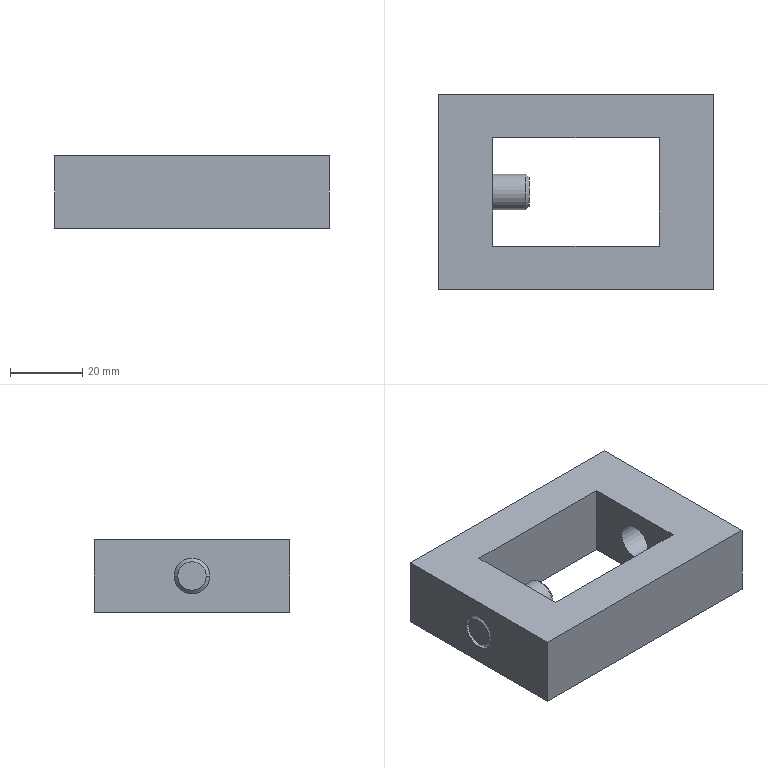Part | SolidWorks | features MirrorStock 1 | 2 solids | 22 faces | box 76 x 54 x 20 mm | volume 53995 mm3 | plane 12 | cylinder 6 | cone 4 | commonest cylinder face diameters 9.9 x4 10.2 x2
STEP:
#1=CARTESIAN_POINT('',(23.,0.,-5.1));
#2=VERTEX_POINT('',#1);
#3=CARTESIAN_POINT('',(23.,0.,5.1));
#4=VERTEX_POINT('',#3);
#5=CARTESIAN_POINT('',(23.,0.,0.));
#6=DIRECTION('',(1.,0.,0.));
#7=DIRECTION('',(0.,0.,-1.));
#8=AXIS2_PLACEMENT_3D('',#5,#6,#7);
#9=CIRCLE('',#8,5.1);
#10=EDGE_CURVE('',#2,#4,#9,.T.);
#11=ORIENTED_EDGE('',*,*,#10,.F.);
#12=CARTESIAN_POINT('',(38.,0.,-5.1));
#13=VERTEX_POINT('',#12);
#14=CARTESIAN_POINT('',(38.,0.,-5.1));
#15=DIRECTION('',(1.,0.,0.));
#16=VECTOR('',#15,1000.);
#17=LINE('',#14,#16);
#18=EDGE_CURVE('',#2,#13,#17,.T.);
#19=ORIENTED_EDGE('',*,*,#18,.T.);
#20=CARTESIAN_POINT('',(38.,0.,5.1));
#21=VERTEX_POINT('',#20);
#22=CARTESIAN_POINT('',(38.,0.,0.));
#23=DIRECTION('',(-1.,0.,0.));
#24=DIRECTION('',(0.,0.,1.));
#25=AXIS2_PLACEMENT_3D('',#22,#23,#24);
#26=CIRCLE('',#25,5.1);
#27=EDGE_CURVE('',#21,#13,#26,.T.);
#28=ORIENTED_EDGE('',*,*,#27,.F.);
#29=CARTESIAN_POINT('',(38.,0.,5.1));
#30=DIRECTION('',(1.,0.,0.));
#31=VECTOR('',#30,1000.);
#32=LINE('',#29,#31);
#33=EDGE_CURVE('',#4,#21,#32,.T.);
#34=ORIENTED_EDGE('',*,*,#33,.F.);
#35=EDGE_LOOP('',(#11,#19,#28,#34));
#36=FACE_OUTER_BOUND('',#35,.T.);
#37=CARTESIAN_POINT('',(38.,0.,0.));
#38=DIRECTION('',(1.,0.,0.));
#39=DIRECTION('',(0.,0.,1.));
#40=AXIS2_PLACEMENT_3D('',#37,#38,#39);
#41=CYLINDRICAL_SURFACE('',#40,5.1);
#42=ADVANCED_FACE('',(#36),#41,.F.);
#43=CARTESIAN_POINT('',(-23.,4.95,0.));
#44=VERTEX_POINT('',#43);
#45=CARTESIAN_POINT('',(-23.,-4.95,0.));
#46=VERTEX_POINT('',#45);
#47=CARTESIAN_POINT('',(-23.,0.,0.));
#48=DIRECTION('',(-1.,0.,0.));
#49=DIRECTION('',(0.,0.,1.));
#50=AXIS2_PLACEMENT_3D('',#47,#48,#49);
#51=CIRCLE('',#50,4.95);
#52=EDGE_CURVE('',#44,#46,#51,.T.);
#53=ORIENTED_EDGE('',*,*,#52,.F.);
#54=CARTESIAN_POINT('',(-38.,4.95,0.));
#55=VERTEX_POINT('',#54);
#56=CARTESIAN_POINT('',(-18.,4.95,0.));
#57=DIRECTION('',(-1.,0.,0.));
#58=VECTOR('',#57,1000.);
#59=LINE('',#56,#58);
#60=EDGE_CURVE('',#44,#55,#59,.T.);
#61=ORIENTED_EDGE('',*,*,#60,.T.);
#62=CARTESIAN_POINT('',(-38.,-4.95,0.));
#63=VERTEX_POINT('',#62);
#64=CARTESIAN_POINT('',(-38.,0.,0.));
#65=DIRECTION('',(1.,0.,0.));
#66=DIRECTION('',(0.,-1.,0.));
#67=AXIS2_PLACEMENT_3D('',#64,#65,#66);
#68=CIRCLE('',#67,4.95);
#69=EDGE_CURVE('',#63,#55,#68,.T.);
#70=ORIENTED_EDGE('',*,*,#69,.F.);
#71=CARTESIAN_POINT('',(-18.,-4.95,0.));
#72=DIRECTION('',(-1.,0.,0.));
#73=VECTOR('',#72,1000.);
#74=LINE('',#71,#73);
#75=EDGE_CURVE('',#46,#63,#74,.T.);
#76=ORIENTED_EDGE('',*,*,#75,.F.);
#77=EDGE_LOOP('',(#53,#61,#70,#76));
#78=FACE_OUTER_BOUND('',#77,.T.);
#79=CARTESIAN_POINT('',(-18.,0.,0.));
#80=DIRECTION('',(-1.,0.,0.));
#81=DIRECTION('',(0.,-1.,0.));
#82=AXIS2_PLACEMENT_3D('',#79,#80,#81);
#83=CYLINDRICAL_SURFACE('',#82,4.95);
#84=ADVANCED_FACE('',(#78),#83,.F.);
#85=CARTESIAN_POINT('',(38.,-27.,-10.));
#86=VERTEX_POINT('',#85);
#87=CARTESIAN_POINT('',(38.,27.,-10.));
#88=VERTEX_POINT('',#87);
#89=CARTESIAN_POINT('',(38.,-27.,-10.));
#90=DIRECTION('',(0.,1.,0.));
#91=VECTOR('',#90,1000.);
#92=LINE('',#89,#91);
#93=EDGE_CURVE('',#86,#88,#92,.T.);
#94=ORIENTED_EDGE('',*,*,#93,.F.);
#95=CARTESIAN_POINT('',(-38.,-27.,-10.));
#96=VERTEX_POINT('',#95);
#97=CARTESIAN_POINT('',(-38.,-27.,-10.));
#98=DIRECTION('',(1.,0.,0.));
#99=VECTOR('',#98,1000.);
#100=LINE('',#97,#99);
#101=EDGE_CURVE('',#96,#86,#100,.T.);
#102=ORIENTED_EDGE('',*,*,#101,.F.);
#103=CARTESIAN_POINT('',(-38.,27.,-10.));
#104=VERTEX_POINT('',#103);
#105=CARTESIAN_POINT('',(-38.,-27.,-10.));
#106=DIRECTION('',(0.,-1.,0.));
#107=VECTOR('',#106,1000.);
#108=LINE('',#105,#107);
#109=EDGE_CURVE('',#104,#96,#108,.T.);
#110=ORIENTED_EDGE('',*,*,#109,.F.);
#111=CARTESIAN_POINT('',(-38.,27.,-10.));
#112=DIRECTION('',(-1.,0.,0.));
#113=VECTOR('',#112,1000.);
#114=LINE('',#111,#113);
#115=EDGE_CURVE('',#88,#104,#114,.T.);
#116=ORIENTED_EDGE('',*,*,#115,.F.);
#117=EDGE_LOOP('',(#94,#102,#110,#116));
#118=FACE_OUTER_BOUND('',#117,.T.);
#119=CARTESIAN_POINT('',(-23.,15.,-10.));
#120=VERTEX_POINT('',#119);
#121=CARTESIAN_POINT('',(-23.,-15.,-10.));
#122=VERTEX_POINT('',#121);
#123=CARTESIAN_POINT('',(-23.,15.,-10.));
#124=DIRECTION('',(0.,-1.,0.));
#125=VECTOR('',#124,1000.);
#126=LINE('',#123,#125);
#127=EDGE_CURVE('',#120,#122,#126,.T.);
#128=ORIENTED_EDGE('',*,*,#127,.T.);
#129=CARTESIAN_POINT('',(23.,-15.,-10.));
#130=VERTEX_POINT('',#129);
#131=CARTESIAN_POINT('',(23.,-15.,-10.));
#132=DIRECTION('',(1.,0.,0.));
#133=VECTOR('',#132,1000.);
#134=LINE('',#131,#133);
#135=EDGE_CURVE('',#122,#130,#134,.T.);
#136=ORIENTED_EDGE('',*,*,#135,.T.);
#137=CARTESIAN_POINT('',(23.,15.,-10.));
#138=VERTEX_POINT('',#137);
#139=CARTESIAN_POINT('',(23.,15.,-10.));
#140=DIRECTION('',(0.,1.,0.));
#141=VECTOR('',#140,1000.);
#142=LINE('',#139,#141);
#143=EDGE_CURVE('',#130,#138,#142,.T.);
#144=ORIENTED_EDGE('',*,*,#143,.T.);
#145=CARTESIAN_POINT('',(23.,15.,-10.));
#146=DIRECTION('',(-1.,0.,0.));
#147=VECTOR('',#146,1000.);
#148=LINE('',#145,#147);
#149=EDGE_CURVE('',#138,#120,#148,.T.);
#150=ORIENTED_EDGE('',*,*,#149,.T.);
#151=EDGE_LOOP('',(#128,#136,#144,#150));
#152=FACE_BOUND('',#151,.T.);
#153=CARTESIAN_POINT('',(0.,0.,-10.));
#154=DIRECTION('',(0.,0.,1.));
#155=DIRECTION('',(-1.,0.,0.));
#156=AXIS2_PLACEMENT_3D('',#153,#154,#155);
#157=PLANE('',#156);
#158=ADVANCED_FACE('',(#118,#152),#157,.F.);
#159=CARTESIAN_POINT('',(38.,-27.,10.));
#160=VERTEX_POINT('',#159);
#161=CARTESIAN_POINT('',(38.,27.,10.));
#162=VERTEX_POINT('',#161);
#163=CARTESIAN_POINT('',(38.,-27.,10.));
#164=DIRECTION('',(0.,1.,0.));
#165=VECTOR('',#164,1000.);
#166=LINE('',#163,#165);
#167=EDGE_CURVE('',#160,#162,#166,.T.);
#168=ORIENTED_EDGE('',*,*,#167,.T.);
#169=CARTESIAN_POINT('',(-38.,27.,10.));
#170=VERTEX_POINT('',#169);
#171=CARTESIAN_POINT('',(-38.,27.,10.));
#172=DIRECTION('',(-1.,0.,0.));
#173=VECTOR('',#172,1000.);
#174=LINE('',#171,#173);
#175=EDGE_CURVE('',#162,#170,#174,.T.);
#176=ORIENTED_EDGE('',*,*,#175,.T.);
#177=CARTESIAN_POINT('',(-38.,-27.,10.));
#178=VERTEX_POINT('',#177);
#179=CARTESIAN_POINT('',(-38.,-27.,10.));
#180=DIRECTION('',(0.,-1.,0.));
#181=VECTOR('',#180,1000.);
#182=LINE('',#179,#181);
#183=EDGE_CURVE('',#170,#178,#182,.T.);
#184=ORIENTED_EDGE('',*,*,#183,.T.);
#185=CARTESIAN_POINT('',(-38.,-27.,10.));
#186=DIRECTION('',(1.,0.,0.));
#187=VECTOR('',#186,1000.);
#188=LINE('',#185,#187);
#189=EDGE_CURVE('',#178,#160,#188,.T.);
#190=ORIENTED_EDGE('',*,*,#189,.T.);
#191=EDGE_LOOP('',(#168,#176,#184,#190));
#192=FACE_OUTER_BOUND('',#191,.T.);
#193=CARTESIAN_POINT('',(23.,15.,10.));
#194=VERTEX_POINT('',#193);
#195=CARTESIAN_POINT('',(-23.,15.,10.));
#196=VERTEX_POINT('',#195);
#197=CARTESIAN_POINT('',(23.,15.,10.));
#198=DIRECTION('',(-1.,0.,0.));
#199=VECTOR('',#198,1000.);
#200=LINE('',#197,#199);
#201=EDGE_CURVE('',#194,#196,#200,.T.);
#202=ORIENTED_EDGE('',*,*,#201,.F.);
#203=CARTESIAN_POINT('',(23.,-15.,10.));
#204=VERTEX_POINT('',#203);
#205=CARTESIAN_POINT('',(23.,15.,10.));
#206=DIRECTION('',(0.,1.,0.));
#207=VECTOR('',#206,1000.);
#208=LINE('',#205,#207);
#209=EDGE_CURVE('',#204,#194,#208,.T.);
#210=ORIENTED_EDGE('',*,*,#209,.F.);
#211=CARTESIAN_POINT('',(-23.,-15.,10.));
#212=VERTEX_POINT('',#211);
#213=CARTESIAN_POINT('',(23.,-15.,10.));
#214=DIRECTION('',(1.,0.,0.));
#215=VECTOR('',#214,1000.);
#216=LINE('',#213,#215);
#217=EDGE_CURVE('',#212,#204,#216,.T.);
#218=ORIENTED_EDGE('',*,*,#217,.F.);
#219=CARTESIAN_POINT('',(-23.,15.,10.));
#220=DIRECTION('',(0.,-1.,0.));
#221=VECTOR('',#220,1000.);
#222=LINE('',#219,#221);
#223=EDGE_CURVE('',#196,#212,#222,.T.);
#224=ORIENTED_EDGE('',*,*,#223,.F.);
#225=EDGE_LOOP('',(#202,#210,#218,#224));
#226=FACE_BOUND('',#225,.T.);
#227=CARTESIAN_POINT('',(0.,0.,10.));
#228=DIRECTION('',(0.,0.,1.));
#229=DIRECTION('',(-1.,0.,0.));
#230=AXIS2_PLACEMENT_3D('',#227,#228,#229);
#231=PLANE('',#230);
#232=ADVANCED_FACE('',(#192,#226),#231,.T.);
#233=ORIENTED_EDGE('',*,*,#27,.T.);
#234=CARTESIAN_POINT('',(38.,0.,0.));
#235=DIRECTION('',(-1.,0.,0.));
#236=DIRECTION('',(0.,0.,1.));
#237=AXIS2_PLACEMENT_3D('',#234,#235,#236);
#238=CIRCLE('',#237,5.1);
#239=EDGE_CURVE('',#13,#21,#238,.T.);
#240=ORIENTED_EDGE('',*,*,#239,.T.);
#241=EDGE_LOOP('',(#233,#240));
#242=FACE_BOUND('',#241,.T.);
#243=ORIENTED_EDGE('',*,*,#167,.F.);
#244=CARTESIAN_POINT('',(38.,-27.,-10.));
#245=DIRECTION('',(0.,0.,1.));
#246=VECTOR('',#245,1000.);
#247=LINE('',#244,#246);
#248=EDGE_CURVE('',#86,#160,#247,.T.);
#249=ORIENTED_EDGE('',*,*,#248,.F.);
#250=ORIENTED_EDGE('',*,*,#93,.T.);
#251=CARTESIAN_POINT('',(38.,27.,-10.));
#252=DIRECTION('',(0.,0.,1.));
#253=VECTOR('',#252,1000.);
#254=LINE('',#251,#253);
#255=EDGE_CURVE('',#88,#162,#254,.T.);
#256=ORIENTED_EDGE('',*,*,#255,.T.);
#257=EDGE_LOOP('',(#243,#249,#250,#256));
#258=FACE_OUTER_BOUND('',#257,.T.);
#259=CARTESIAN_POINT('',(38.,-27.,-10.));
#260=DIRECTION('',(-1.,0.,0.));
#261=DIRECTION('',(0.,-1.,0.));
#262=AXIS2_PLACEMENT_3D('',#259,#260,#261);
#263=PLANE('',#262);
#264=ADVANCED_FACE('',(#242,#258),#263,.F.);
#265=ORIENTED_EDGE('',*,*,#175,.F.);
#266=ORIENTED_EDGE('',*,*,#255,.F.);
#267=ORIENTED_EDGE('',*,*,#115,.T.);
#268=CARTESIAN_POINT('',(-38.,27.,-10.));
#269=DIRECTION('',(0.,0.,1.));
#270=VECTOR('',#269,1000.);
#271=LINE('',#268,#270);
#272=EDGE_CURVE('',#104,#170,#271,.T.);
#273=ORIENTED_EDGE('',*,*,#272,.T.);
#274=EDGE_LOOP('',(#265,#266,#267,#273));
#275=FACE_OUTER_BOUND('',#274,.T.);
#276=CARTESIAN_POINT('',(-38.,27.,-10.));
#277=DIRECTION('',(0.,-1.,0.));
#278=DIRECTION('',(1.,0.,0.));
#279=AXIS2_PLACEMENT_3D('',#276,#277,#278);
#280=PLANE('',#279);
#281=ADVANCED_FACE('',(#275),#280,.F.);
#282=ORIENTED_EDGE('',*,*,#69,.T.);
#283=CARTESIAN_POINT('',(-38.,0.,0.));
#284=DIRECTION('',(1.,0.,0.));
#285=DIRECTION('',(0.,-1.,0.));
#286=AXIS2_PLACEMENT_3D('',#283,#284,#285);
#287=CIRCLE('',#286,4.95);
#288=EDGE_CURVE('',#55,#63,#287,.T.);
#289=ORIENTED_EDGE('',*,*,#288,.T.);
#290=EDGE_LOOP('',(#282,#289));
#291=FACE_BOUND('',#290,.T.);
#292=ORIENTED_EDGE('',*,*,#183,.F.);
#293=ORIENTED_EDGE('',*,*,#272,.F.);
#294=ORIENTED_EDGE('',*,*,#109,.T.);
#295=CARTESIAN_POINT('',(-38.,-27.,-10.));
#296=DIRECTION('',(0.,0.,1.));
#297=VECTOR('',#296,1000.);
#298=LINE('',#295,#297);
#299=EDGE_CURVE('',#96,#178,#298,.T.);
#300=ORIENTED_EDGE('',*,*,#299,.T.);
#301=EDGE_LOOP('',(#292,#293,#294,#300));
#302=FACE_OUTER_BOUND('',#301,.T.);
#303=CARTESIAN_POINT('',(-38.,-27.,-10.));
#304=DIRECTION('',(1.,0.,0.));
#305=DIRECTION('',(0.,1.,0.));
#306=AXIS2_PLACEMENT_3D('',#303,#304,#305);
#307=PLANE('',#306);
#308=ADVANCED_FACE('',(#291,#302),#307,.F.);
#309=ORIENTED_EDGE('',*,*,#189,.F.);
#310=ORIENTED_EDGE('',*,*,#299,.F.);
#311=ORIENTED_EDGE('',*,*,#101,.T.);
#312=ORIENTED_EDGE('',*,*,#248,.T.);
#313=EDGE_LOOP('',(#309,#310,#311,#312));
#314=FACE_OUTER_BOUND('',#313,.T.);
#315=CARTESIAN_POINT('',(-38.,-27.,-10.));
#316=DIRECTION('',(0.,1.,0.));
#317=DIRECTION('',(-1.,0.,0.));
#318=AXIS2_PLACEMENT_3D('',#315,#316,#317);
#319=PLANE('',#318);
#320=ADVANCED_FACE('',(#314),#319,.F.);
#321=CARTESIAN_POINT('',(-23.,0.,0.));
#322=DIRECTION('',(-1.,0.,0.));
#323=DIRECTION('',(0.,0.,1.));
#324=AXIS2_PLACEMENT_3D('',#321,#322,#323);
#325=CIRCLE('',#324,4.95);
#326=EDGE_CURVE('',#46,#44,#325,.T.);
#327=ORIENTED_EDGE('',*,*,#326,.T.);
#328=ORIENTED_EDGE('',*,*,#52,.T.);
#329=EDGE_LOOP('',(#327,#328));
#330=FACE_BOUND('',#329,.T.);
#331=ORIENTED_EDGE('',*,*,#223,.T.);
#332=CARTESIAN_POINT('',(-23.,-15.,-10.));
#333=DIRECTION('',(0.,0.,1.));
#334=VECTOR('',#333,1000.);
#335=LINE('',#332,#334);
#336=EDGE_CURVE('',#122,#212,#335,.T.);
#337=ORIENTED_EDGE('',*,*,#336,.F.);
#338=ORIENTED_EDGE('',*,*,#127,.F.);
#339=CARTESIAN_POINT('',(-23.,15.,-10.));
#340=DIRECTION('',(0.,0.,1.));
#341=VECTOR('',#340,1000.);
#342=LINE('',#339,#341);
#343=EDGE_CURVE('',#120,#196,#342,.T.);
#344=ORIENTED_EDGE('',*,*,#343,.T.);
#345=EDGE_LOOP('',(#331,#337,#338,#344));
#346=FACE_OUTER_BOUND('',#345,.T.);
#347=CARTESIAN_POINT('',(-23.,15.,-10.));
#348=DIRECTION('',(1.,0.,0.));
#349=DIRECTION('',(0.,0.,1.));
#350=AXIS2_PLACEMENT_3D('',#347,#348,#349);
#351=PLANE('',#350);
#352=ADVANCED_FACE('',(#330,#346),#351,.T.);
#353=ORIENTED_EDGE('',*,*,#217,.T.);
#354=CARTESIAN_POINT('',(23.,-15.,-10.));
#355=DIRECTION('',(0.,0.,1.));
#356=VECTOR('',#355,1000.);
#357=LINE('',#354,#356);
#358=EDGE_CURVE('',#130,#204,#357,.T.);
#359=ORIENTED_EDGE('',*,*,#358,.F.);
#360=ORIENTED_EDGE('',*,*,#135,.F.);
#361=ORIENTED_EDGE('',*,*,#336,.T.);
#362=EDGE_LOOP('',(#353,#359,#360,#361));
#363=FACE_OUTER_BOUND('',#362,.T.);
#364=CARTESIAN_POINT('',(23.,-15.,-10.));
#365=DIRECTION('',(0.,1.,0.));
#366=DIRECTION('',(0.,0.,-1.));
#367=AXIS2_PLACEMENT_3D('',#364,#365,#366);
#368=PLANE('',#367);
#369=ADVANCED_FACE('',(#363),#368,.T.);
#370=CARTESIAN_POINT('',(23.,0.,0.));
#371=DIRECTION('',(1.,0.,0.));
#372=DIRECTION('',(0.,0.,-1.));
#373=AXIS2_PLACEMENT_3D('',#370,#371,#372);
#374=CIRCLE('',#373,5.1);
#375=EDGE_CURVE('',#4,#2,#374,.T.);
#376=ORIENTED_EDGE('',*,*,#375,.T.);
#377=ORIENTED_EDGE('',*,*,#10,.T.);
#378=EDGE_LOOP('',(#376,#377));
#379=FACE_BOUND('',#378,.T.);
#380=ORIENTED_EDGE('',*,*,#209,.T.);
#381=CARTESIAN_POINT('',(23.,15.,-10.));
#382=DIRECTION('',(0.,0.,1.));
#383=VECTOR('',#382,1000.);
#384=LINE('',#381,#383);
#385=EDGE_CURVE('',#138,#194,#384,.T.);
#386=ORIENTED_EDGE('',*,*,#385,.F.);
#387=ORIENTED_EDGE('',*,*,#143,.F.);
#388=ORIENTED_EDGE('',*,*,#358,.T.);
#389=EDGE_LOOP('',(#380,#386,#387,#388));
#390=FACE_OUTER_BOUND('',#389,.T.);
#391=CARTESIAN_POINT('',(23.,15.,-10.));
#392=DIRECTION('',(-1.,0.,0.));
#393=DIRECTION('',(0.,0.,-1.));
#394=AXIS2_PLACEMENT_3D('',#391,#392,#393);
#395=PLANE('',#394);
#396=ADVANCED_FACE('',(#379,#390),#395,.T.);
#397=ORIENTED_EDGE('',*,*,#201,.T.);
#398=ORIENTED_EDGE('',*,*,#343,.F.);
#399=ORIENTED_EDGE('',*,*,#149,.F.);
#400=ORIENTED_EDGE('',*,*,#385,.T.);
#401=EDGE_LOOP('',(#397,#398,#399,#400));
#402=FACE_OUTER_BOUND('',#401,.T.);
#403=CARTESIAN_POINT('',(23.,15.,-10.));
#404=DIRECTION('',(0.,-1.,0.));
#405=DIRECTION('',(1.,0.,0.));
#406=AXIS2_PLACEMENT_3D('',#403,#404,#405);
#407=PLANE('',#406);
#408=ADVANCED_FACE('',(#402),#407,.T.);
#409=ORIENTED_EDGE('',*,*,#60,.F.);
#410=ORIENTED_EDGE('',*,*,#326,.F.);
#411=ORIENTED_EDGE('',*,*,#75,.T.);
#412=ORIENTED_EDGE('',*,*,#288,.F.);
#413=EDGE_LOOP('',(#409,#410,#411,#412));
#414=FACE_OUTER_BOUND('',#413,.T.);
#415=CARTESIAN_POINT('',(-18.,0.,0.));
#416=DIRECTION('',(-1.,0.,0.));
#417=DIRECTION('',(0.,-1.,0.));
#418=AXIS2_PLACEMENT_3D('',#415,#416,#417);
#419=CYLINDRICAL_SURFACE('',#418,4.95);
#420=ADVANCED_FACE('',(#414),#419,.F.);
#421=ORIENTED_EDGE('',*,*,#18,.F.);
#422=ORIENTED_EDGE('',*,*,#375,.F.);
#423=ORIENTED_EDGE('',*,*,#33,.T.);
#424=ORIENTED_EDGE('',*,*,#239,.F.);
#425=EDGE_LOOP('',(#421,#422,#423,#424));
#426=FACE_OUTER_BOUND('',#425,.T.);
#427=CARTESIAN_POINT('',(38.,0.,0.));
#428=DIRECTION('',(1.,0.,0.));
#429=DIRECTION('',(0.,0.,1.));
#430=AXIS2_PLACEMENT_3D('',#427,#428,#429);
#431=CYLINDRICAL_SURFACE('',#430,5.1);
#432=ADVANCED_FACE('',(#426),#431,.F.);
#433=CLOSED_SHELL('',(#42,#84,#158,#232,#264,#281,#308,#320,#352,#369,#396,#408,#420,#432));
#434=MANIFOLD_SOLID_BREP('',#433);
#435=CARTESIAN_POINT('',(-13.,-3.95,0.));
#436=VERTEX_POINT('',#435);
#437=CARTESIAN_POINT('',(-13.,3.95,0.));
#438=VERTEX_POINT('',#437);
#439=CARTESIAN_POINT('',(-13.,0.,0.));
#440=DIRECTION('',(-1.,0.,0.));
#441=DIRECTION('',(0.,-1.,0.));
#442=AXIS2_PLACEMENT_3D('',#439,#440,#441);
#443=CIRCLE('',#442,3.95);
#444=EDGE_CURVE('',#436,#438,#443,.T.);
#445=ORIENTED_EDGE('',*,*,#444,.T.);
#446=CARTESIAN_POINT('',(-14.,4.95,0.));
#447=VERTEX_POINT('',#446);
#448=CARTESIAN_POINT('',(-14.,4.95,0.));
#449=DIRECTION('',(-0.7071,0.7071,0.));
#450=VECTOR('',#449,1000.);
#451=LINE('',#448,#450);
#452=EDGE_CURVE('',#438,#447,#451,.T.);
#453=ORIENTED_EDGE('',*,*,#452,.T.);
#454=CARTESIAN_POINT('',(-14.,-4.95,0.));
#455=VERTEX_POINT('',#454);
#456=CARTESIAN_POINT('',(-14.,0.,0.));
#457=DIRECTION('',(1.,0.,0.));
#458=DIRECTION('',(0.,-1.,0.));
#459=AXIS2_PLACEMENT_3D('',#456,#457,#458);
#460=CIRCLE('',#459,4.95);
#461=EDGE_CURVE('',#447,#455,#460,.T.);
#462=ORIENTED_EDGE('',*,*,#461,.T.);
#463=CARTESIAN_POINT('',(-14.,-4.95,0.));
#464=DIRECTION('',(-0.7071,-0.7071,0.));
#465=VECTOR('',#464,1000.);
#466=LINE('',#463,#465);
#467=EDGE_CURVE('',#436,#455,#466,.T.);
#468=ORIENTED_EDGE('',*,*,#467,.F.);
#469=EDGE_LOOP('',(#445,#453,#462,#468));
#470=FACE_OUTER_BOUND('',#469,.T.);
#471=CARTESIAN_POINT('',(-14.,0.,0.));
#472=DIRECTION('',(-1.,0.,0.));
#473=DIRECTION('',(0.,-1.,0.));
#474=AXIS2_PLACEMENT_3D('',#471,#472,#473);
#475=CONICAL_SURFACE('',#474,4.95,0.7854);
#476=ADVANCED_FACE('',(#470),#475,.T.);
#477=CARTESIAN_POINT('',(-38.,3.95,0.));
#478=VERTEX_POINT('',#477);
#479=CARTESIAN_POINT('',(-38.,-3.95,0.));
#480=VERTEX_POINT('',#479);
#481=CARTESIAN_POINT('',(-38.,0.,0.));
#482=DIRECTION('',(1.,0.,0.));
#483=DIRECTION('',(0.,-1.,0.));
#484=AXIS2_PLACEMENT_3D('',#481,#482,#483);
#485=CIRCLE('',#484,3.95);
#486=EDGE_CURVE('',#478,#480,#485,.T.);
#487=ORIENTED_EDGE('',*,*,#486,.T.);
#488=CARTESIAN_POINT('',(-37.,-4.95,0.));
#489=VERTEX_POINT('',#488);
#490=CARTESIAN_POINT('',(-38.,-3.95,0.));
#491=DIRECTION('',(0.7071,-0.7071,0.));
#492=VECTOR('',#491,1000.);
#493=LINE('',#490,#492);
#494=EDGE_CURVE('',#480,#489,#493,.T.);
#495=ORIENTED_EDGE('',*,*,#494,.T.);
#496=CARTESIAN_POINT('',(-37.,4.95,0.));
#497=VERTEX_POINT('',#496);
#498=CARTESIAN_POINT('',(-37.,0.,0.));
#499=DIRECTION('',(-1.,0.,0.));
#500=DIRECTION('',(0.,-1.,0.));
#501=AXIS2_PLACEMENT_3D('',#498,#499,#500);
#502=CIRCLE('',#501,4.95);
#503=EDGE_CURVE('',#489,#497,#502,.T.);
#504=ORIENTED_EDGE('',*,*,#503,.T.);
#505=CARTESIAN_POINT('',(-38.,3.95,0.));
#506=DIRECTION('',(0.7071,0.7071,0.));
#507=VECTOR('',#506,1000.);
#508=LINE('',#505,#507);
#509=EDGE_CURVE('',#478,#497,#508,.T.);
#510=ORIENTED_EDGE('',*,*,#509,.F.);
#511=EDGE_LOOP('',(#487,#495,#504,#510));
#512=FACE_OUTER_BOUND('',#511,.T.);
#513=CARTESIAN_POINT('',(-38.,0.,0.));
#514=DIRECTION('',(1.,0.,0.));
#515=DIRECTION('',(0.,1.,0.));
#516=AXIS2_PLACEMENT_3D('',#513,#514,#515);
#517=CONICAL_SURFACE('',#516,3.95,0.7854);
#518=ADVANCED_FACE('',(#512),#517,.T.);
#519=ORIENTED_EDGE('',*,*,#461,.F.);
#520=CARTESIAN_POINT('',(-13.,4.95,0.));
#521=DIRECTION('',(-1.,0.,0.));
#522=VECTOR('',#521,1000.);
#523=LINE('',#520,#522);
#524=EDGE_CURVE('',#447,#497,#523,.T.);
#525=ORIENTED_EDGE('',*,*,#524,.T.);
#526=ORIENTED_EDGE('',*,*,#503,.F.);
#527=CARTESIAN_POINT('',(-13.,-4.95,0.));
#528=DIRECTION('',(-1.,0.,0.));
#529=VECTOR('',#528,1000.);
#530=LINE('',#527,#529);
#531=EDGE_CURVE('',#455,#489,#530,.T.);
#532=ORIENTED_EDGE('',*,*,#531,.F.);
#533=EDGE_LOOP('',(#519,#525,#526,#532));
#534=FACE_OUTER_BOUND('',#533,.T.);
#535=CARTESIAN_POINT('',(-13.,0.,0.));
#536=DIRECTION('',(-1.,0.,0.));
#537=DIRECTION('',(0.,-1.,0.));
#538=AXIS2_PLACEMENT_3D('',#535,#536,#537);
#539=CYLINDRICAL_SURFACE('',#538,4.95);
#540=ADVANCED_FACE('',(#534),#539,.T.);
#541=ORIENTED_EDGE('',*,*,#524,.F.);
#542=CARTESIAN_POINT('',(-14.,0.,0.));
#543=DIRECTION('',(1.,0.,0.));
#544=DIRECTION('',(0.,-1.,0.));
#545=AXIS2_PLACEMENT_3D('',#542,#543,#544);
#546=CIRCLE('',#545,4.95);
#547=EDGE_CURVE('',#455,#447,#546,.T.);
#548=ORIENTED_EDGE('',*,*,#547,.F.);
#549=ORIENTED_EDGE('',*,*,#531,.T.);
#550=CARTESIAN_POINT('',(-37.,0.,0.));
#551=DIRECTION('',(-1.,0.,0.));
#552=DIRECTION('',(0.,-1.,0.));
#553=AXIS2_PLACEMENT_3D('',#550,#551,#552);
#554=CIRCLE('',#553,4.95);
#555=EDGE_CURVE('',#497,#489,#554,.T.);
#556=ORIENTED_EDGE('',*,*,#555,.F.);
#557=EDGE_LOOP('',(#541,#548,#549,#556));
#558=FACE_OUTER_BOUND('',#557,.T.);
#559=CARTESIAN_POINT('',(-13.,0.,0.));
#560=DIRECTION('',(-1.,0.,0.));
#561=DIRECTION('',(0.,-1.,0.));
#562=AXIS2_PLACEMENT_3D('',#559,#560,#561);
#563=CYLINDRICAL_SURFACE('',#562,4.95);
#564=ADVANCED_FACE('',(#558),#563,.T.);
#565=ORIENTED_EDGE('',*,*,#444,.F.);
#566=CARTESIAN_POINT('',(-13.,0.,0.));
#567=DIRECTION('',(-1.,0.,0.));
#568=DIRECTION('',(0.,-1.,0.));
#569=AXIS2_PLACEMENT_3D('',#566,#567,#568);
#570=CIRCLE('',#569,3.95);
#571=EDGE_CURVE('',#438,#436,#570,.T.);
#572=ORIENTED_EDGE('',*,*,#571,.F.);
#573=EDGE_LOOP('',(#565,#572));
#574=FACE_OUTER_BOUND('',#573,.T.);
#575=CARTESIAN_POINT('',(-13.,0.,0.));
#576=DIRECTION('',(-1.,0.,0.));
#577=DIRECTION('',(0.,-1.,0.));
#578=AXIS2_PLACEMENT_3D('',#575,#576,#577);
#579=PLANE('',#578);
#580=ADVANCED_FACE('',(#574),#579,.F.);
#581=ORIENTED_EDGE('',*,*,#486,.F.);
#582=CARTESIAN_POINT('',(-38.,0.,0.));
#583=DIRECTION('',(1.,0.,0.));
#584=DIRECTION('',(0.,-1.,0.));
#585=AXIS2_PLACEMENT_3D('',#582,#583,#584);
#586=CIRCLE('',#585,3.95);
#587=EDGE_CURVE('',#480,#478,#586,.T.);
#588=ORIENTED_EDGE('',*,*,#587,.F.);
#589=EDGE_LOOP('',(#581,#588));
#590=FACE_OUTER_BOUND('',#589,.T.);
#591=CARTESIAN_POINT('',(-38.,0.,0.));
#592=DIRECTION('',(-1.,0.,0.));
#593=DIRECTION('',(0.,-1.,0.));
#594=AXIS2_PLACEMENT_3D('',#591,#592,#593);
#595=PLANE('',#594);
#596=ADVANCED_FACE('',(#590),#595,.T.);
#597=ORIENTED_EDGE('',*,*,#494,.F.);
#598=ORIENTED_EDGE('',*,*,#587,.T.);
#599=ORIENTED_EDGE('',*,*,#509,.T.);
#600=ORIENTED_EDGE('',*,*,#555,.T.);
#601=EDGE_LOOP('',(#597,#598,#599,#600));
#602=FACE_OUTER_BOUND('',#601,.T.);
#603=CARTESIAN_POINT('',(-38.,0.,0.));
#604=DIRECTION('',(1.,0.,0.));
#605=DIRECTION('',(0.,1.,0.));
#606=AXIS2_PLACEMENT_3D('',#603,#604,#605);
#607=CONICAL_SURFACE('',#606,3.95,0.7854);
#608=ADVANCED_FACE('',(#602),#607,.T.);
#609=ORIENTED_EDGE('',*,*,#452,.F.);
#610=ORIENTED_EDGE('',*,*,#571,.T.);
#611=ORIENTED_EDGE('',*,*,#467,.T.);
#612=ORIENTED_EDGE('',*,*,#547,.T.);
#613=EDGE_LOOP('',(#609,#610,#611,#612));
#614=FACE_OUTER_BOUND('',#613,.T.);
#615=CARTESIAN_POINT('',(-14.,0.,0.));
#616=DIRECTION('',(-1.,0.,0.));
#617=DIRECTION('',(0.,-1.,0.));
#618=AXIS2_PLACEMENT_3D('',#615,#616,#617);
#619=CONICAL_SURFACE('',#618,4.95,0.7854);
#620=ADVANCED_FACE('',(#614),#619,.T.);
#621=CLOSED_SHELL('',(#476,#518,#540,#564,#580,#596,#608,#620));
#622=MANIFOLD_SOLID_BREP('',#621);
#623=CARTESIAN_POINT('',(0.,0.,0.));
#624=DIRECTION('',(0.,0.,1.));
#625=DIRECTION('',(1.,0.,0.));
#626=AXIS2_PLACEMENT_3D('',#623,#624,#625);
#627=(LENGTH_UNIT()NAMED_UNIT(*)SI_UNIT(.MILLI.,.METRE.));
#628=UNCERTAINTY_MEASURE_WITH_UNIT(LENGTH_MEASURE(0.00001),#627,'','');
#629=(NAMED_UNIT(*)PLANE_ANGLE_UNIT()SI_UNIT($,.RADIAN.));
#630=(NAMED_UNIT(*)SI_UNIT($,.STERADIAN.)SOLID_ANGLE_UNIT());
#631=(GEOMETRIC_REPRESENTATION_CONTEXT(3)GLOBAL_UNCERTAINTY_ASSIGNED_CONTEXT((#628))GLOBAL_UNIT_ASSIGNED_CONTEXT((#627,#629,#630))REPRESENTATION_CONTEXT('',''));
#632=ADVANCED_BREP_SHAPE_REPRESENTATION('',(#434,#622,#626),#631);